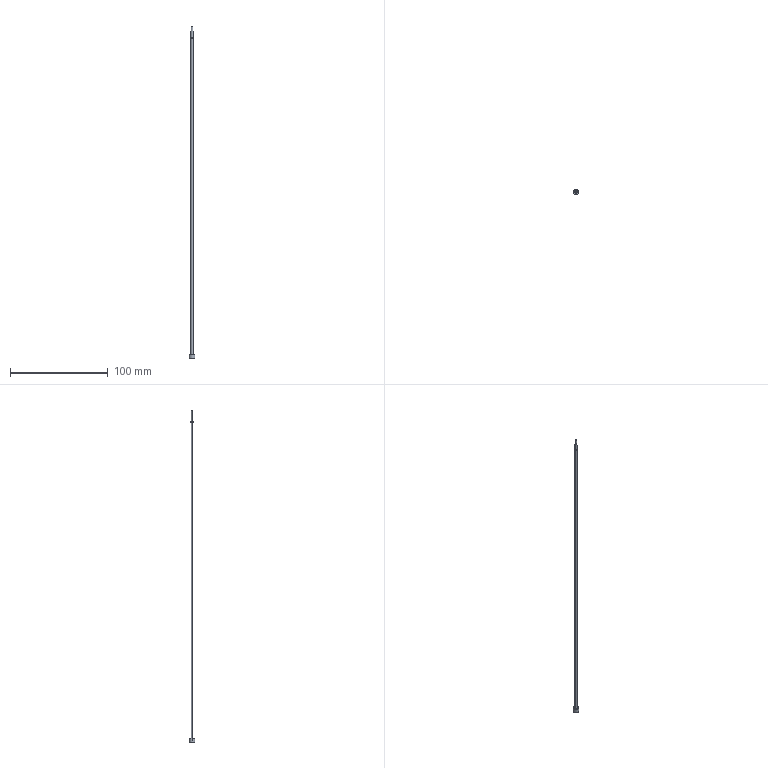Part | Creo | 1 solid | 13 faces | box 6 x 6 x 339.575 mm | volume 2146 mm3 | plane 5 | cone 4 | cylinder 4 | commonest cylinder face diameters 2.8 x2 6 x2
STEP:
#1=CARTESIAN_POINT('',(49.138,-56.28,-20.728));
#2=VERTEX_POINT('',#1);
#3=CARTESIAN_POINT('',(46.338,-56.28,-20.728));
#4=VERTEX_POINT('',#3);
#5=CARTESIAN_POINT('',(47.738,-56.28,-20.728));
#6=DIRECTION('',(0.,0.,1.));
#7=DIRECTION('',(1.,0.,0.));
#8=AXIS2_PLACEMENT_3D('',#5,#6,#7);
#9=CIRCLE('',#8,1.4);
#10=EDGE_CURVE('',#2,#4,#9,.T.);
#11=ORIENTED_EDGE('',*,*,#10,.F.);
#12=CARTESIAN_POINT('',(47.738,-56.28,-20.728));
#13=DIRECTION('',(0.,0.,1.));
#14=DIRECTION('',(-1.,0.,0.));
#15=AXIS2_PLACEMENT_3D('',#12,#13,#14);
#16=CIRCLE('',#15,1.4);
#17=EDGE_CURVE('',#4,#2,#16,.T.);
#18=ORIENTED_EDGE('',*,*,#17,.F.);
#19=EDGE_LOOP('',(#11,#18));
#20=FACE_OUTER_BOUND('',#19,.F.);
#21=CARTESIAN_POINT('',(49.1,-56.28,-20.728));
#22=VERTEX_POINT('',#21);
#23=CARTESIAN_POINT('',(46.375,-56.28,-20.728));
#24=VERTEX_POINT('',#23);
#25=CARTESIAN_POINT('',(47.737,-56.28,-20.728));
#26=DIRECTION('',(0.,0.,-1.));
#27=DIRECTION('',(1.,0.,0.));
#28=AXIS2_PLACEMENT_3D('',#25,#26,#27);
#29=CIRCLE('',#28,1.362);
#30=EDGE_CURVE('',#22,#24,#29,.T.);
#31=ORIENTED_EDGE('',*,*,#30,.F.);
#32=CARTESIAN_POINT('',(47.737,-56.28,-20.728));
#33=DIRECTION('',(0.,0.,-1.));
#34=DIRECTION('',(-1.,0.,0.));
#35=AXIS2_PLACEMENT_3D('',#32,#33,#34);
#36=CIRCLE('',#35,1.362);
#37=EDGE_CURVE('',#24,#22,#36,.T.);
#38=ORIENTED_EDGE('',*,*,#37,.F.);
#39=EDGE_LOOP('',(#31,#38));
#40=FACE_BOUND('',#39,.F.);
#41=CARTESIAN_POINT('',(47.737,-56.318,-20.728));
#42=DIRECTION('',(0.,0.,1.));
#43=DIRECTION('',(1.,0.,0.));
#44=AXIS2_PLACEMENT_3D('',#41,#42,#43);
#45=PLANE('',#44);
#46=ADVANCED_FACE('',(#20,#40),#45,.T.);
#47=CARTESIAN_POINT('',(46.389,-56.28,-19.924));
#48=VERTEX_POINT('',#47);
#49=CARTESIAN_POINT('',(49.086,-56.28,-19.924));
#50=VERTEX_POINT('',#49);
#51=CARTESIAN_POINT('',(47.737,-56.28,-19.924));
#52=DIRECTION('',(0.,0.,1.));
#53=DIRECTION('',(-1.,0.,0.));
#54=AXIS2_PLACEMENT_3D('',#51,#52,#53);
#55=CIRCLE('',#54,1.348);
#56=EDGE_CURVE('',#48,#50,#55,.T.);
#57=ORIENTED_EDGE('',*,*,#56,.T.);
#58=CARTESIAN_POINT('',(49.086,-56.28,-19.924));
#59=DIRECTION('',(0.01745,0.,-0.9998));
#60=VECTOR('',#59,0.8041);
#61=LINE('',#58,#60);
#62=EDGE_CURVE('',#50,#22,#61,.T.);
#63=ORIENTED_EDGE('',*,*,#62,.T.);
#64=ORIENTED_EDGE('',*,*,#30,.T.);
#65=CARTESIAN_POINT('',(46.389,-56.28,-19.924));
#66=DIRECTION('',(-0.01745,0.,-0.9998));
#67=VECTOR('',#66,0.8041);
#68=LINE('',#65,#67);
#69=EDGE_CURVE('',#48,#24,#68,.T.);
#70=ORIENTED_EDGE('',*,*,#69,.F.);
#71=EDGE_LOOP('',(#57,#63,#64,#70));
#72=FACE_OUTER_BOUND('',#71,.F.);
#73=CARTESIAN_POINT('',(47.737,-56.28,-20.326));
#74=DIRECTION('',(0.,0.,-1.));
#75=DIRECTION('',(1.,0.,0.));
#76=AXIS2_PLACEMENT_3D('',#73,#74,#75);
#77=CONICAL_SURFACE('',#76,1.355,1.);
#78=ADVANCED_FACE('',(#72),#77,.T.);
#79=ORIENTED_EDGE('',*,*,#56,.F.);
#80=CARTESIAN_POINT('',(47.737,-56.28,-19.924));
#81=DIRECTION('',(0.,0.,1.));
#82=DIRECTION('',(1.,0.,0.));
#83=AXIS2_PLACEMENT_3D('',#80,#81,#82);
#84=CIRCLE('',#83,1.348);
#85=EDGE_CURVE('',#50,#48,#84,.T.);
#86=ORIENTED_EDGE('',*,*,#85,.F.);
#87=EDGE_LOOP('',(#79,#86));
#88=FACE_OUTER_BOUND('',#87,.F.);
#89=CARTESIAN_POINT('',(46.656,-56.28,-19.924));
#90=VERTEX_POINT('',#89);
#91=CARTESIAN_POINT('',(48.819,-56.28,-19.924));
#92=VERTEX_POINT('',#91);
#93=CARTESIAN_POINT('',(47.737,-56.28,-19.924));
#94=DIRECTION('',(0.,0.,-1.));
#95=DIRECTION('',(-1.,0.,0.));
#96=AXIS2_PLACEMENT_3D('',#93,#94,#95);
#97=CIRCLE('',#96,1.081);
#98=EDGE_CURVE('',#90,#92,#97,.T.);
#99=ORIENTED_EDGE('',*,*,#98,.F.);
#100=CARTESIAN_POINT('',(47.737,-56.28,-19.924));
#101=DIRECTION('',(0.,0.,-1.));
#102=DIRECTION('',(1.,0.,0.));
#103=AXIS2_PLACEMENT_3D('',#100,#101,#102);
#104=CIRCLE('',#103,1.081);
#105=EDGE_CURVE('',#92,#90,#104,.T.);
#106=ORIENTED_EDGE('',*,*,#105,.F.);
#107=EDGE_LOOP('',(#99,#106));
#108=FACE_BOUND('',#107,.F.);
#109=CARTESIAN_POINT('',(47.737,-56.28,-19.924));
#110=DIRECTION('',(0.,0.,-1.));
#111=DIRECTION('',(-1.,0.,0.));
#112=AXIS2_PLACEMENT_3D('',#109,#110,#111);
#113=PLANE('',#112);
#114=ADVANCED_FACE('',(#88,#108),#113,.F.);
#115=CARTESIAN_POINT('',(46.757,-56.28,-8.425));
#116=VERTEX_POINT('',#115);
#117=CARTESIAN_POINT('',(48.718,-56.28,-8.459));
#118=VERTEX_POINT('',#117);
#119=CARTESIAN_POINT('',(46.757,-56.28,-8.425));
#120=CARTESIAN_POINT('',(46.757,-56.049,-8.425));
#121=CARTESIAN_POINT('',(46.969,-55.499,-8.429));
#122=CARTESIAN_POINT('',(47.738,-55.199,-8.442));
#123=CARTESIAN_POINT('',(48.506,-55.499,-8.456));
#124=CARTESIAN_POINT('',(48.718,-56.049,-8.459));
#125=CARTESIAN_POINT('',(48.718,-56.28,-8.459));
#126=B_SPLINE_CURVE_WITH_KNOTS('',3,(#119,#120,#121,#122,#123,#124,#125),.UNSPECIFIED.,.F.,.F.,(4,1,1,1,4),(0.,0.25,0.5,0.75,1.),.UNSPECIFIED.);
#127=EDGE_CURVE('',#116,#118,#126,.T.);
#128=ORIENTED_EDGE('',*,*,#127,.F.);
#129=CARTESIAN_POINT('',(46.757,-56.28,-8.425));
#130=DIRECTION('',(-0.008727,0.,-1.));
#131=VECTOR('',#130,11.499);
#132=LINE('',#129,#131);
#133=EDGE_CURVE('',#116,#90,#132,.T.);
#134=ORIENTED_EDGE('',*,*,#133,.T.);
#135=ORIENTED_EDGE('',*,*,#98,.T.);
#136=CARTESIAN_POINT('',(48.718,-56.28,-8.459));
#137=DIRECTION('',(0.008727,0.,-1.));
#138=VECTOR('',#137,11.465);
#139=LINE('',#136,#138);
#140=EDGE_CURVE('',#118,#92,#139,.T.);
#141=ORIENTED_EDGE('',*,*,#140,.F.);
#142=EDGE_LOOP('',(#128,#134,#135,#141));
#143=FACE_OUTER_BOUND('',#142,.F.);
#144=CARTESIAN_POINT('',(47.737,-56.28,-14.175));
#145=DIRECTION('',(0.,0.,-1.));
#146=DIRECTION('',(-1.,0.,0.));
#147=AXIS2_PLACEMENT_3D('',#144,#145,#146);
#148=CONICAL_SURFACE('',#147,1.031,0.5);
#149=ADVANCED_FACE('',(#143),#148,.T.);
#150=ORIENTED_EDGE('',*,*,#127,.T.);
#151=CARTESIAN_POINT('',(48.718,-56.28,-8.459));
#152=CARTESIAN_POINT('',(48.718,-56.511,-8.459));
#153=CARTESIAN_POINT('',(48.506,-57.061,-8.456));
#154=CARTESIAN_POINT('',(47.738,-57.361,-8.442));
#155=CARTESIAN_POINT('',(46.969,-57.061,-8.429));
#156=CARTESIAN_POINT('',(46.757,-56.511,-8.425));
#157=CARTESIAN_POINT('',(46.757,-56.28,-8.425));
#158=B_SPLINE_CURVE_WITH_KNOTS('',3,(#151,#152,#153,#154,#155,#156,#157),.UNSPECIFIED.,.F.,.F.,(4,1,1,1,4),(0.,0.25,0.5,0.75,1.),.UNSPECIFIED.);
#159=EDGE_CURVE('',#118,#116,#158,.T.);
#160=ORIENTED_EDGE('',*,*,#159,.T.);
#161=EDGE_LOOP('',(#150,#160));
#162=FACE_OUTER_BOUND('',#161,.F.);
#163=CARTESIAN_POINT('',(60.807,-51.758,-8.67));
#164=DIRECTION('',(-0.01745,0.,-0.9998));
#165=DIRECTION('',(-0.9998,0.,0.01745));
#166=AXIS2_PLACEMENT_3D('',#163,#164,#165);
#167=PLANE('',#166);
#168=ADVANCED_FACE('',(#162),#167,.F.);
#169=ORIENTED_EDGE('',*,*,#159,.F.);
#170=ORIENTED_EDGE('',*,*,#140,.T.);
#171=ORIENTED_EDGE('',*,*,#105,.T.);
#172=ORIENTED_EDGE('',*,*,#133,.F.);
#173=EDGE_LOOP('',(#169,#170,#171,#172));
#174=FACE_OUTER_BOUND('',#173,.F.);
#175=CARTESIAN_POINT('',(47.737,-56.28,-14.175));
#176=DIRECTION('',(0.,0.,-1.));
#177=DIRECTION('',(-1.,0.,0.));
#178=AXIS2_PLACEMENT_3D('',#175,#176,#177);
#179=CONICAL_SURFACE('',#178,1.031,0.5);
#180=ADVANCED_FACE('',(#174),#179,.T.);
#181=ORIENTED_EDGE('',*,*,#85,.T.);
#182=ORIENTED_EDGE('',*,*,#69,.T.);
#183=ORIENTED_EDGE('',*,*,#37,.T.);
#184=ORIENTED_EDGE('',*,*,#62,.F.);
#185=EDGE_LOOP('',(#181,#182,#183,#184));
#186=FACE_OUTER_BOUND('',#185,.F.);
#187=CARTESIAN_POINT('',(47.737,-56.28,-20.326));
#188=DIRECTION('',(0.,0.,-1.));
#189=DIRECTION('',(1.,0.,0.));
#190=AXIS2_PLACEMENT_3D('',#187,#188,#189);
#191=CONICAL_SURFACE('',#190,1.355,1.);
#192=ADVANCED_FACE('',(#186),#191,.T.);
#193=CARTESIAN_POINT('',(46.338,-56.28,-344.));
#194=VERTEX_POINT('',#193);
#195=CARTESIAN_POINT('',(49.138,-56.28,-344.));
#196=VERTEX_POINT('',#195);
#197=CARTESIAN_POINT('',(47.738,-56.28,-344.));
#198=DIRECTION('',(0.,0.,-1.));
#199=DIRECTION('',(-1.,0.,0.));
#200=AXIS2_PLACEMENT_3D('',#197,#198,#199);
#201=CIRCLE('',#200,1.4);
#202=EDGE_CURVE('',#194,#196,#201,.T.);
#203=ORIENTED_EDGE('',*,*,#202,.T.);
#204=CARTESIAN_POINT('',(49.138,-56.28,-344.));
#205=DIRECTION('',(0.,0.,1.));
#206=VECTOR('',#205,323.272);
#207=LINE('',#204,#206);
#208=EDGE_CURVE('',#196,#2,#207,.T.);
#209=ORIENTED_EDGE('',*,*,#208,.T.);
#210=ORIENTED_EDGE('',*,*,#10,.T.);
#211=CARTESIAN_POINT('',(46.338,-56.28,-344.));
#212=DIRECTION('',(0.,0.,1.));
#213=VECTOR('',#212,323.272);
#214=LINE('',#211,#213);
#215=EDGE_CURVE('',#194,#4,#214,.T.);
#216=ORIENTED_EDGE('',*,*,#215,.F.);
#217=EDGE_LOOP('',(#203,#209,#210,#216));
#218=FACE_OUTER_BOUND('',#217,.F.);
#219=CARTESIAN_POINT('',(47.738,-56.28,-428.));
#220=DIRECTION('',(0.,0.,1.));
#221=DIRECTION('',(1.,0.,0.));
#222=AXIS2_PLACEMENT_3D('',#219,#220,#221);
#223=CYLINDRICAL_SURFACE('',#222,1.4);
#224=ADVANCED_FACE('',(#218),#223,.T.);
#225=CARTESIAN_POINT('',(50.738,-56.28,-344.));
#226=VERTEX_POINT('',#225);
#227=CARTESIAN_POINT('',(44.738,-56.28,-344.));
#228=VERTEX_POINT('',#227);
#229=CARTESIAN_POINT('',(47.738,-56.28,-344.));
#230=DIRECTION('',(0.,0.,1.));
#231=DIRECTION('',(1.,0.,0.));
#232=AXIS2_PLACEMENT_3D('',#229,#230,#231);
#233=CIRCLE('',#232,3.);
#234=EDGE_CURVE('',#226,#228,#233,.T.);
#235=ORIENTED_EDGE('',*,*,#234,.F.);
#236=CARTESIAN_POINT('',(47.738,-56.28,-344.));
#237=DIRECTION('',(0.,0.,1.));
#238=DIRECTION('',(-1.,0.,0.));
#239=AXIS2_PLACEMENT_3D('',#236,#237,#238);
#240=CIRCLE('',#239,3.);
#241=EDGE_CURVE('',#228,#226,#240,.T.);
#242=ORIENTED_EDGE('',*,*,#241,.F.);
#243=EDGE_LOOP('',(#235,#242));
#244=FACE_OUTER_BOUND('',#243,.F.);
#245=CARTESIAN_POINT('',(47.738,-56.28,-344.));
#246=DIRECTION('',(0.,0.,-1.));
#247=DIRECTION('',(1.,0.,0.));
#248=AXIS2_PLACEMENT_3D('',#245,#246,#247);
#249=CIRCLE('',#248,1.4);
#250=EDGE_CURVE('',#196,#194,#249,.T.);
#251=ORIENTED_EDGE('',*,*,#250,.F.);
#252=ORIENTED_EDGE('',*,*,#202,.F.);
#253=EDGE_LOOP('',(#251,#252));
#254=FACE_BOUND('',#253,.F.);
#255=CARTESIAN_POINT('',(47.738,-56.28,-344.));
#256=DIRECTION('',(0.,0.,1.));
#257=DIRECTION('',(1.,0.,0.));
#258=AXIS2_PLACEMENT_3D('',#255,#256,#257);
#259=PLANE('',#258);
#260=ADVANCED_FACE('',(#244,#254),#259,.T.);
#261=ORIENTED_EDGE('',*,*,#250,.T.);
#262=ORIENTED_EDGE('',*,*,#215,.T.);
#263=ORIENTED_EDGE('',*,*,#17,.T.);
#264=ORIENTED_EDGE('',*,*,#208,.F.);
#265=EDGE_LOOP('',(#261,#262,#263,#264));
#266=FACE_OUTER_BOUND('',#265,.F.);
#267=CARTESIAN_POINT('',(47.738,-56.28,-428.));
#268=DIRECTION('',(0.,0.,1.));
#269=DIRECTION('',(1.,0.,0.));
#270=AXIS2_PLACEMENT_3D('',#267,#268,#269);
#271=CYLINDRICAL_SURFACE('',#270,1.4);
#272=ADVANCED_FACE('',(#266),#271,.T.);
#273=ORIENTED_EDGE('',*,*,#234,.T.);
#274=CARTESIAN_POINT('',(44.738,-56.28,-348.));
#275=VERTEX_POINT('',#274);
#276=CARTESIAN_POINT('',(44.738,-56.28,-348.));
#277=DIRECTION('',(0.,0.,1.));
#278=VECTOR('',#277,4.);
#279=LINE('',#276,#278);
#280=EDGE_CURVE('',#275,#228,#279,.T.);
#281=ORIENTED_EDGE('',*,*,#280,.F.);
#282=CARTESIAN_POINT('',(50.738,-56.28,-348.));
#283=VERTEX_POINT('',#282);
#284=CARTESIAN_POINT('',(47.738,-56.28,-348.));
#285=DIRECTION('',(0.,0.,-1.));
#286=DIRECTION('',(-1.,0.,0.));
#287=AXIS2_PLACEMENT_3D('',#284,#285,#286);
#288=CIRCLE('',#287,3.);
#289=EDGE_CURVE('',#275,#283,#288,.T.);
#290=ORIENTED_EDGE('',*,*,#289,.T.);
#291=CARTESIAN_POINT('',(50.738,-56.28,-348.));
#292=DIRECTION('',(0.,0.,1.));
#293=VECTOR('',#292,4.);
#294=LINE('',#291,#293);
#295=EDGE_CURVE('',#283,#226,#294,.T.);
#296=ORIENTED_EDGE('',*,*,#295,.T.);
#297=EDGE_LOOP('',(#273,#281,#290,#296));
#298=FACE_OUTER_BOUND('',#297,.F.);
#299=CARTESIAN_POINT('',(47.738,-56.28,-348.));
#300=DIRECTION('',(0.,0.,1.));
#301=DIRECTION('',(1.,0.,0.));
#302=AXIS2_PLACEMENT_3D('',#299,#300,#301);
#303=CYLINDRICAL_SURFACE('',#302,3.);
#304=ADVANCED_FACE('',(#298),#303,.T.);
#305=ORIENTED_EDGE('',*,*,#241,.T.);
#306=ORIENTED_EDGE('',*,*,#295,.F.);
#307=CARTESIAN_POINT('',(47.738,-56.28,-348.));
#308=DIRECTION('',(0.,0.,-1.));
#309=DIRECTION('',(1.,0.,0.));
#310=AXIS2_PLACEMENT_3D('',#307,#308,#309);
#311=CIRCLE('',#310,3.);
#312=EDGE_CURVE('',#283,#275,#311,.T.);
#313=ORIENTED_EDGE('',*,*,#312,.T.);
#314=ORIENTED_EDGE('',*,*,#280,.T.);
#315=EDGE_LOOP('',(#305,#306,#313,#314));
#316=FACE_OUTER_BOUND('',#315,.F.);
#317=CARTESIAN_POINT('',(47.738,-56.28,-348.));
#318=DIRECTION('',(0.,0.,1.));
#319=DIRECTION('',(1.,0.,0.));
#320=AXIS2_PLACEMENT_3D('',#317,#318,#319);
#321=CYLINDRICAL_SURFACE('',#320,3.);
#322=ADVANCED_FACE('',(#316),#321,.T.);
#323=ORIENTED_EDGE('',*,*,#312,.F.);
#324=ORIENTED_EDGE('',*,*,#289,.F.);
#325=EDGE_LOOP('',(#323,#324));
#326=FACE_OUTER_BOUND('',#325,.F.);
#327=CARTESIAN_POINT('',(68.,-62.005,-348.));
#328=DIRECTION('',(0.,0.,1.));
#329=DIRECTION('',(1.,0.,0.));
#330=AXIS2_PLACEMENT_3D('',#327,#328,#329);
#331=PLANE('',#330);
#332=ADVANCED_FACE('',(#326),#331,.F.);
#333=CLOSED_SHELL('',(#46,#78,#114,#149,#168,#180,#192,#224,#260,#272,#304,#322,#332));
#334=MANIFOLD_SOLID_BREP('',#333);
#335=(LENGTH_UNIT()NAMED_UNIT(*)SI_UNIT(.MILLI.,.METRE.));
#336=UNCERTAINTY_MEASURE_WITH_UNIT(LENGTH_MEASURE(0.03397),#335,'','');
#337=(NAMED_UNIT(*)PLANE_ANGLE_UNIT()SI_UNIT($,.RADIAN.));
#338=PLANE_ANGLE_MEASURE_WITH_UNIT(PLANE_ANGLE_MEASURE(0.01745),#337);
#339=(CONVERSION_BASED_UNIT('DEGREE',#338)NAMED_UNIT(*)PLANE_ANGLE_UNIT());
#340=(NAMED_UNIT(*)SI_UNIT($,.STERADIAN.)SOLID_ANGLE_UNIT());
#341=(GEOMETRIC_REPRESENTATION_CONTEXT(3)GLOBAL_UNCERTAINTY_ASSIGNED_CONTEXT((#336))GLOBAL_UNIT_ASSIGNED_CONTEXT((#335,#339,#340))REPRESENTATION_CONTEXT('',''));
#342=ADVANCED_BREP_SHAPE_REPRESENTATION('',(#334),#341);